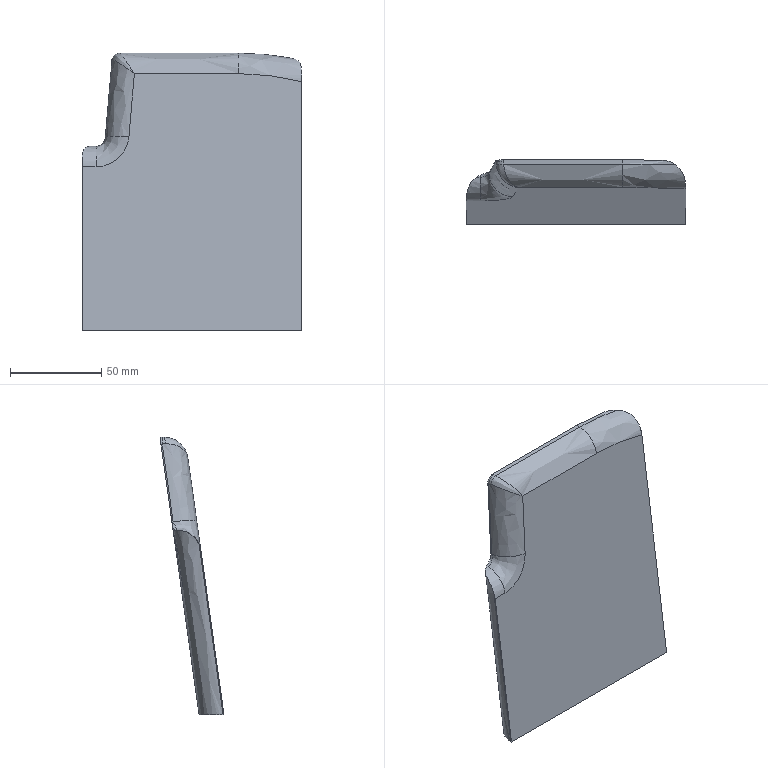Part | STEP file | solid 55 | 1 solid | 20 faces | box 120 x 34.962 x 151.763 mm | volume 223888 mm3 | spline 11 | plane 5 | cylinder 3 | other 1 | commonest cylinder face diameters 8.104 x1 10.13 x1 303.9 x1